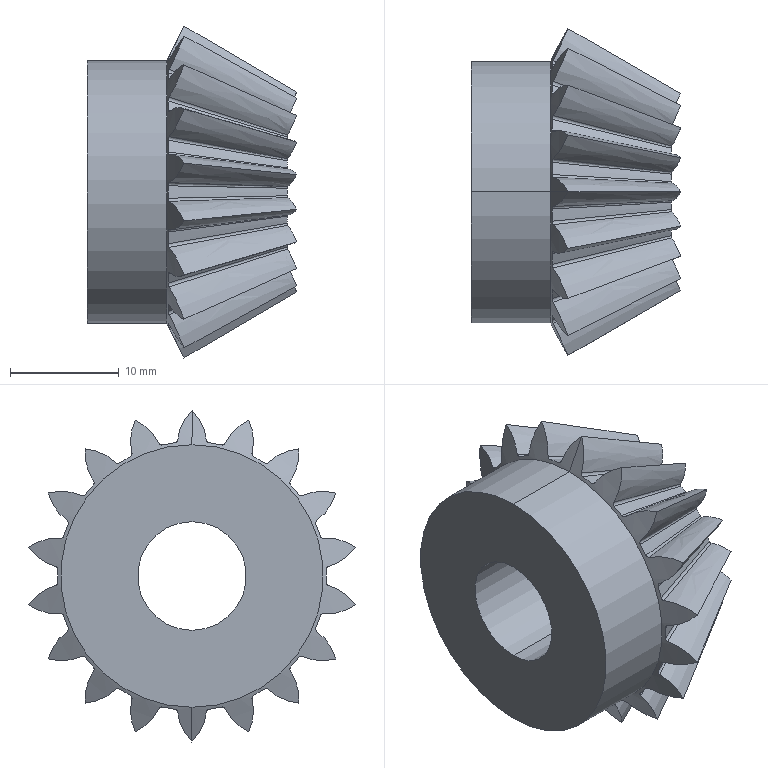Part | SolidWorks | features CirPattern 2, Cut 2, BlendCut 1, Boss 1, ICE 1, Revolution 1 | 1 solid | 100 faces | box 19.27 x 30.102 x 30.566 mm | volume 6238 mm3 | spline 90 | cylinder 4 | cone 4 | plane 2 | commonest cylinder face diameters 10 x2 24.17 x2